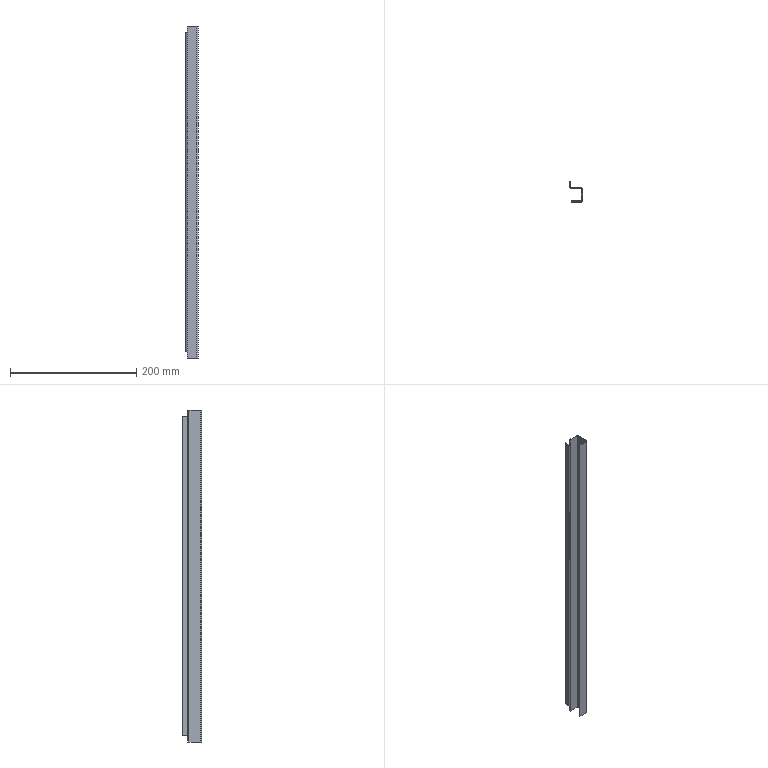Part | SolidWorks | features EdgeFlange 1, FlatPattern 1, SMBaseFlange 1, SheetMetal 1 | 1 solid | 32 faces | box 19.1 x 31.2 x 525 mm | volume 39715 mm3 | plane 26 | cylinder 6 | commonest cylinder face diameters 1.4 x3 3.8 x3
STEP:
#1=CARTESIAN_POINT('',(0.,21.2,262.5));
#2=VERTEX_POINT('',#1);
#3=CARTESIAN_POINT('',(0.,21.2,252.5));
#4=VERTEX_POINT('',#3);
#5=CARTESIAN_POINT('',(0.,21.2,262.5));
#6=DIRECTION('',(0.,0.,-1.));
#7=VECTOR('',#6,1000.);
#8=LINE('',#5,#7);
#9=EDGE_CURVE('',#2,#4,#8,.T.);
#10=ORIENTED_EDGE('',*,*,#9,.T.);
#11=CARTESIAN_POINT('',(0.,20.,252.5));
#12=VERTEX_POINT('',#11);
#13=CARTESIAN_POINT('',(0.,21.2,252.5));
#14=DIRECTION('',(0.,-1.,0.));
#15=VECTOR('',#14,1000.);
#16=LINE('',#13,#15);
#17=EDGE_CURVE('',#4,#12,#16,.T.);
#18=ORIENTED_EDGE('',*,*,#17,.T.);
#19=CARTESIAN_POINT('',(0.,20.,262.5));
#20=VERTEX_POINT('',#19);
#21=CARTESIAN_POINT('',(0.,20.,262.5));
#22=DIRECTION('',(0.,0.,-1.));
#23=VECTOR('',#22,1000.);
#24=LINE('',#21,#23);
#25=EDGE_CURVE('',#20,#12,#24,.T.);
#26=ORIENTED_EDGE('',*,*,#25,.F.);
#27=CARTESIAN_POINT('',(0.,20.,262.5));
#28=DIRECTION('',(0.,1.,0.));
#29=VECTOR('',#28,1000.);
#30=LINE('',#27,#29);
#31=EDGE_CURVE('',#20,#2,#30,.T.);
#32=ORIENTED_EDGE('',*,*,#31,.T.);
#33=EDGE_LOOP('',(#10,#18,#26,#32));
#34=FACE_OUTER_BOUND('',#33,.T.);
#35=CARTESIAN_POINT('',(0.,20.,262.5));
#36=DIRECTION('',(-1.,0.,0.));
#37=DIRECTION('',(0.,0.,1.));
#38=AXIS2_PLACEMENT_3D('',#35,#36,#37);
#39=PLANE('',#38);
#40=ADVANCED_FACE('',(#34),#39,.T.);
#41=CARTESIAN_POINT('',(16.,0.7,262.5));
#42=VERTEX_POINT('',#41);
#43=CARTESIAN_POINT('',(17.2,0.7,262.5));
#44=VERTEX_POINT('',#43);
#45=CARTESIAN_POINT('',(16.,0.7,262.5));
#46=DIRECTION('',(1.,0.,0.));
#47=VECTOR('',#46,1000.);
#48=LINE('',#45,#47);
#49=EDGE_CURVE('',#42,#44,#48,.T.);
#50=ORIENTED_EDGE('',*,*,#49,.F.);
#51=CARTESIAN_POINT('',(15.3,0.,262.5));
#52=VERTEX_POINT('',#51);
#53=CARTESIAN_POINT('',(15.3,0.7,262.5));
#54=DIRECTION('',(0.,0.,1.));
#55=DIRECTION('',(-1.,0.,0.));
#56=AXIS2_PLACEMENT_3D('',#53,#54,#55);
#57=CIRCLE('',#56,0.7);
#58=EDGE_CURVE('',#52,#42,#57,.T.);
#59=ORIENTED_EDGE('',*,*,#58,.F.);
#60=CARTESIAN_POINT('',(15.3,-1.2,262.5));
#61=VERTEX_POINT('',#60);
#62=CARTESIAN_POINT('',(15.3,-1.2,262.5));
#63=DIRECTION('',(0.,1.,0.));
#64=VECTOR('',#63,1000.);
#65=LINE('',#62,#64);
#66=EDGE_CURVE('',#61,#52,#65,.T.);
#67=ORIENTED_EDGE('',*,*,#66,.F.);
#68=CARTESIAN_POINT('',(15.3,0.7,262.5));
#69=DIRECTION('',(0.,0.,1.));
#70=DIRECTION('',(1.,0.,0.));
#71=AXIS2_PLACEMENT_3D('',#68,#69,#70);
#72=CIRCLE('',#71,1.9);
#73=EDGE_CURVE('',#61,#44,#72,.T.);
#74=ORIENTED_EDGE('',*,*,#73,.T.);
#75=EDGE_LOOP('',(#50,#59,#67,#74));
#76=FACE_OUTER_BOUND('',#75,.T.);
#77=CARTESIAN_POINT('',(16.,0.7,262.5));
#78=DIRECTION('',(0.,0.,1.));
#79=DIRECTION('',(1.,0.,0.));
#80=AXIS2_PLACEMENT_3D('',#77,#78,#79);
#81=PLANE('',#80);
#82=ADVANCED_FACE('',(#76),#81,.T.);
#83=CARTESIAN_POINT('',(16.,19.3,262.5));
#84=VERTEX_POINT('',#83);
#85=CARTESIAN_POINT('',(16.,0.,262.5));
#86=DIRECTION('',(0.,1.,0.));
#87=VECTOR('',#86,1000.);
#88=LINE('',#85,#87);
#89=EDGE_CURVE('',#42,#84,#88,.T.);
#90=ORIENTED_EDGE('',*,*,#89,.F.);
#91=ORIENTED_EDGE('',*,*,#49,.T.);
#92=CARTESIAN_POINT('',(17.2,19.3,262.5));
#93=VERTEX_POINT('',#92);
#94=CARTESIAN_POINT('',(17.2,0.,262.5));
#95=DIRECTION('',(0.,1.,0.));
#96=VECTOR('',#95,1000.);
#97=LINE('',#94,#96);
#98=EDGE_CURVE('',#44,#93,#97,.T.);
#99=ORIENTED_EDGE('',*,*,#98,.T.);
#100=CARTESIAN_POINT('',(17.2,19.3,262.5));
#101=DIRECTION('',(-1.,0.,0.));
#102=VECTOR('',#101,1000.);
#103=LINE('',#100,#102);
#104=EDGE_CURVE('',#93,#84,#103,.T.);
#105=ORIENTED_EDGE('',*,*,#104,.T.);
#106=EDGE_LOOP('',(#90,#91,#99,#105));
#107=FACE_OUTER_BOUND('',#106,.T.);
#108=CARTESIAN_POINT('',(15.3,-1.2,262.5));
#109=DIRECTION('',(0.,0.,1.));
#110=DIRECTION('',(1.,0.,0.));
#111=AXIS2_PLACEMENT_3D('',#108,#109,#110);
#112=PLANE('',#111);
#113=ADVANCED_FACE('',(#107),#112,.T.);
#114=CARTESIAN_POINT('',(15.3,0.,-262.5));
#115=VERTEX_POINT('',#114);
#116=CARTESIAN_POINT('',(15.3,-1.2,-262.5));
#117=VERTEX_POINT('',#116);
#118=CARTESIAN_POINT('',(15.3,0.,-262.5));
#119=DIRECTION('',(0.,-1.,0.));
#120=VECTOR('',#119,1000.);
#121=LINE('',#118,#120);
#122=EDGE_CURVE('',#115,#117,#121,.T.);
#123=ORIENTED_EDGE('',*,*,#122,.F.);
#124=CARTESIAN_POINT('',(16.,0.7,-262.5));
#125=VERTEX_POINT('',#124);
#126=CARTESIAN_POINT('',(15.3,0.7,-262.5));
#127=DIRECTION('',(0.,0.,1.));
#128=DIRECTION('',(-1.,0.,0.));
#129=AXIS2_PLACEMENT_3D('',#126,#127,#128);
#130=CIRCLE('',#129,0.7);
#131=EDGE_CURVE('',#115,#125,#130,.T.);
#132=ORIENTED_EDGE('',*,*,#131,.T.);
#133=CARTESIAN_POINT('',(17.2,0.7,-262.5));
#134=VERTEX_POINT('',#133);
#135=CARTESIAN_POINT('',(17.2,0.7,-262.5));
#136=DIRECTION('',(-1.,0.,0.));
#137=VECTOR('',#136,1000.);
#138=LINE('',#135,#137);
#139=EDGE_CURVE('',#134,#125,#138,.T.);
#140=ORIENTED_EDGE('',*,*,#139,.F.);
#141=CARTESIAN_POINT('',(15.3,0.7,-262.5));
#142=DIRECTION('',(0.,0.,1.));
#143=DIRECTION('',(1.,0.,0.));
#144=AXIS2_PLACEMENT_3D('',#141,#142,#143);
#145=CIRCLE('',#144,1.9);
#146=EDGE_CURVE('',#117,#134,#145,.T.);
#147=ORIENTED_EDGE('',*,*,#146,.F.);
#148=EDGE_LOOP('',(#123,#132,#140,#147));
#149=FACE_OUTER_BOUND('',#148,.T.);
#150=CARTESIAN_POINT('',(15.3,0.,-262.5));
#151=DIRECTION('',(0.,0.,-1.));
#152=DIRECTION('',(-1.,0.,0.));
#153=AXIS2_PLACEMENT_3D('',#150,#151,#152);
#154=PLANE('',#153);
#155=ADVANCED_FACE('',(#149),#154,.T.);
#156=CARTESIAN_POINT('',(0.,0.,-262.5));
#157=VERTEX_POINT('',#156);
#158=CARTESIAN_POINT('',(0.,0.,-262.5));
#159=DIRECTION('',(1.,0.,0.));
#160=VECTOR('',#159,1000.);
#161=LINE('',#158,#160);
#162=EDGE_CURVE('',#157,#115,#161,.T.);
#163=ORIENTED_EDGE('',*,*,#162,.T.);
#164=ORIENTED_EDGE('',*,*,#122,.T.);
#165=CARTESIAN_POINT('',(0.,-1.2,-262.5));
#166=VERTEX_POINT('',#165);
#167=CARTESIAN_POINT('',(0.,-1.2,-262.5));
#168=DIRECTION('',(1.,0.,0.));
#169=VECTOR('',#168,1000.);
#170=LINE('',#167,#169);
#171=EDGE_CURVE('',#166,#117,#170,.T.);
#172=ORIENTED_EDGE('',*,*,#171,.F.);
#173=CARTESIAN_POINT('',(0.,-1.2,-262.5));
#174=DIRECTION('',(0.,1.,0.));
#175=VECTOR('',#174,1000.);
#176=LINE('',#173,#175);
#177=EDGE_CURVE('',#166,#157,#176,.T.);
#178=ORIENTED_EDGE('',*,*,#177,.T.);
#179=EDGE_LOOP('',(#163,#164,#172,#178));
#180=FACE_OUTER_BOUND('',#179,.T.);
#181=CARTESIAN_POINT('',(17.2,0.7,-262.5));
#182=DIRECTION('',(0.,0.,-1.));
#183=DIRECTION('',(-1.,0.,0.));
#184=AXIS2_PLACEMENT_3D('',#181,#182,#183);
#185=PLANE('',#184);
#186=ADVANCED_FACE('',(#180),#185,.T.);
#187=CARTESIAN_POINT('',(15.3,20.,262.5));
#188=VERTEX_POINT('',#187);
#189=CARTESIAN_POINT('',(15.3,21.2,262.5));
#190=VERTEX_POINT('',#189);
#191=CARTESIAN_POINT('',(15.3,20.,262.5));
#192=DIRECTION('',(0.,1.,0.));
#193=VECTOR('',#192,1000.);
#194=LINE('',#191,#193);
#195=EDGE_CURVE('',#188,#190,#194,.T.);
#196=ORIENTED_EDGE('',*,*,#195,.F.);
#197=CARTESIAN_POINT('',(15.3,19.3,262.5));
#198=DIRECTION('',(0.,0.,1.));
#199=DIRECTION('',(-1.,0.,0.));
#200=AXIS2_PLACEMENT_3D('',#197,#198,#199);
#201=CIRCLE('',#200,0.7);
#202=EDGE_CURVE('',#84,#188,#201,.T.);
#203=ORIENTED_EDGE('',*,*,#202,.F.);
#204=ORIENTED_EDGE('',*,*,#104,.F.);
#205=CARTESIAN_POINT('',(15.3,19.3,262.5));
#206=DIRECTION('',(0.,0.,1.));
#207=DIRECTION('',(1.,0.,0.));
#208=AXIS2_PLACEMENT_3D('',#205,#206,#207);
#209=CIRCLE('',#208,1.9);
#210=EDGE_CURVE('',#93,#190,#209,.T.);
#211=ORIENTED_EDGE('',*,*,#210,.T.);
#212=EDGE_LOOP('',(#196,#203,#204,#211));
#213=FACE_OUTER_BOUND('',#212,.T.);
#214=CARTESIAN_POINT('',(15.3,20.,262.5));
#215=DIRECTION('',(0.,0.,1.));
#216=DIRECTION('',(1.,0.,0.));
#217=AXIS2_PLACEMENT_3D('',#214,#215,#216);
#218=PLANE('',#217);
#219=ADVANCED_FACE('',(#213),#218,.T.);
#220=CARTESIAN_POINT('',(16.,20.,262.5));
#221=DIRECTION('',(-1.,0.,0.));
#222=VECTOR('',#221,1000.);
#223=LINE('',#220,#222);
#224=EDGE_CURVE('',#188,#20,#223,.T.);
#225=ORIENTED_EDGE('',*,*,#224,.F.);
#226=ORIENTED_EDGE('',*,*,#195,.T.);
#227=CARTESIAN_POINT('',(16.,21.2,262.5));
#228=DIRECTION('',(-1.,0.,0.));
#229=VECTOR('',#228,1000.);
#230=LINE('',#227,#229);
#231=EDGE_CURVE('',#190,#2,#230,.T.);
#232=ORIENTED_EDGE('',*,*,#231,.T.);
#233=ORIENTED_EDGE('',*,*,#31,.F.);
#234=EDGE_LOOP('',(#225,#226,#232,#233));
#235=FACE_OUTER_BOUND('',#234,.T.);
#236=CARTESIAN_POINT('',(17.2,19.3,262.5));
#237=DIRECTION('',(0.,0.,1.));
#238=DIRECTION('',(1.,0.,0.));
#239=AXIS2_PLACEMENT_3D('',#236,#237,#238);
#240=PLANE('',#239);
#241=ADVANCED_FACE('',(#235),#240,.T.);
#242=CARTESIAN_POINT('',(16.,19.3,-262.5));
#243=VERTEX_POINT('',#242);
#244=CARTESIAN_POINT('',(17.2,19.3,-262.5));
#245=VERTEX_POINT('',#244);
#246=CARTESIAN_POINT('',(16.,19.3,-262.5));
#247=DIRECTION('',(1.,0.,0.));
#248=VECTOR('',#247,1000.);
#249=LINE('',#246,#248);
#250=EDGE_CURVE('',#243,#245,#249,.T.);
#251=ORIENTED_EDGE('',*,*,#250,.F.);
#252=CARTESIAN_POINT('',(15.3,20.,-262.5));
#253=VERTEX_POINT('',#252);
#254=CARTESIAN_POINT('',(15.3,19.3,-262.5));
#255=DIRECTION('',(0.,0.,1.));
#256=DIRECTION('',(-1.,0.,0.));
#257=AXIS2_PLACEMENT_3D('',#254,#255,#256);
#258=CIRCLE('',#257,0.7);
#259=EDGE_CURVE('',#243,#253,#258,.T.);
#260=ORIENTED_EDGE('',*,*,#259,.T.);
#261=CARTESIAN_POINT('',(15.3,21.2,-262.5));
#262=VERTEX_POINT('',#261);
#263=CARTESIAN_POINT('',(15.3,21.2,-262.5));
#264=DIRECTION('',(0.,-1.,0.));
#265=VECTOR('',#264,1000.);
#266=LINE('',#263,#265);
#267=EDGE_CURVE('',#262,#253,#266,.T.);
#268=ORIENTED_EDGE('',*,*,#267,.F.);
#269=CARTESIAN_POINT('',(15.3,19.3,-262.5));
#270=DIRECTION('',(0.,0.,1.));
#271=DIRECTION('',(1.,0.,0.));
#272=AXIS2_PLACEMENT_3D('',#269,#270,#271);
#273=CIRCLE('',#272,1.9);
#274=EDGE_CURVE('',#245,#262,#273,.T.);
#275=ORIENTED_EDGE('',*,*,#274,.F.);
#276=EDGE_LOOP('',(#251,#260,#268,#275));
#277=FACE_OUTER_BOUND('',#276,.T.);
#278=CARTESIAN_POINT('',(16.,19.3,-262.5));
#279=DIRECTION('',(0.,0.,-1.));
#280=DIRECTION('',(-1.,0.,0.));
#281=AXIS2_PLACEMENT_3D('',#278,#279,#280);
#282=PLANE('',#281);
#283=ADVANCED_FACE('',(#277),#282,.T.);
#284=CARTESIAN_POINT('',(16.,0.,-262.5));
#285=DIRECTION('',(0.,1.,0.));
#286=VECTOR('',#285,1000.);
#287=LINE('',#284,#286);
#288=EDGE_CURVE('',#125,#243,#287,.T.);
#289=ORIENTED_EDGE('',*,*,#288,.T.);
#290=ORIENTED_EDGE('',*,*,#250,.T.);
#291=CARTESIAN_POINT('',(17.2,0.,-262.5));
#292=DIRECTION('',(0.,1.,0.));
#293=VECTOR('',#292,1000.);
#294=LINE('',#291,#293);
#295=EDGE_CURVE('',#134,#245,#294,.T.);
#296=ORIENTED_EDGE('',*,*,#295,.F.);
#297=ORIENTED_EDGE('',*,*,#139,.T.);
#298=EDGE_LOOP('',(#289,#290,#296,#297));
#299=FACE_OUTER_BOUND('',#298,.T.);
#300=CARTESIAN_POINT('',(15.3,21.2,-262.5));
#301=DIRECTION('',(0.,0.,-1.));
#302=DIRECTION('',(-1.,0.,0.));
#303=AXIS2_PLACEMENT_3D('',#300,#301,#302);
#304=PLANE('',#303);
#305=ADVANCED_FACE('',(#299),#304,.T.);
#306=CARTESIAN_POINT('',(0.,21.2,-262.5));
#307=VERTEX_POINT('',#306);
#308=CARTESIAN_POINT('',(16.,21.2,-262.5));
#309=DIRECTION('',(-1.,0.,0.));
#310=VECTOR('',#309,1000.);
#311=LINE('',#308,#310);
#312=EDGE_CURVE('',#262,#307,#311,.T.);
#313=ORIENTED_EDGE('',*,*,#312,.T.);
#314=CARTESIAN_POINT('',(0.,21.2,-252.5));
#315=VERTEX_POINT('',#314);
#316=CARTESIAN_POINT('',(0.,21.2,262.5));
#317=DIRECTION('',(0.,0.,-1.));
#318=VECTOR('',#317,1000.);
#319=LINE('',#316,#318);
#320=EDGE_CURVE('',#315,#307,#319,.T.);
#321=ORIENTED_EDGE('',*,*,#320,.F.);
#322=CARTESIAN_POINT('',(0.,21.2,252.5));
#323=DIRECTION('',(0.,0.,-1.));
#324=VECTOR('',#323,1000.);
#325=LINE('',#322,#324);
#326=EDGE_CURVE('',#4,#315,#325,.T.);
#327=ORIENTED_EDGE('',*,*,#326,.F.);
#328=ORIENTED_EDGE('',*,*,#9,.F.);
#329=ORIENTED_EDGE('',*,*,#231,.F.);
#330=CARTESIAN_POINT('',(15.3,21.2,262.5));
#331=DIRECTION('',(0.,0.,-1.));
#332=VECTOR('',#331,1000.);
#333=LINE('',#330,#332);
#334=EDGE_CURVE('',#190,#262,#333,.T.);
#335=ORIENTED_EDGE('',*,*,#334,.T.);
#336=EDGE_LOOP('',(#313,#321,#327,#328,#329,#335));
#337=FACE_OUTER_BOUND('',#336,.T.);
#338=CARTESIAN_POINT('',(16.,21.2,262.5));
#339=DIRECTION('',(0.,-1.,0.));
#340=DIRECTION('',(0.,0.,-1.));
#341=AXIS2_PLACEMENT_3D('',#338,#339,#340);
#342=PLANE('',#341);
#343=ADVANCED_FACE('',(#337),#342,.F.);
#344=CARTESIAN_POINT('',(0.,20.,-252.5));
#345=VERTEX_POINT('',#344);
#346=CARTESIAN_POINT('',(0.,21.2,-252.5));
#347=DIRECTION('',(0.,-1.,0.));
#348=VECTOR('',#347,1000.);
#349=LINE('',#346,#348);
#350=EDGE_CURVE('',#315,#345,#349,.T.);
#351=ORIENTED_EDGE('',*,*,#350,.F.);
#352=ORIENTED_EDGE('',*,*,#320,.T.);
#353=CARTESIAN_POINT('',(0.,20.,-262.5));
#354=VERTEX_POINT('',#353);
#355=CARTESIAN_POINT('',(0.,20.,-262.5));
#356=DIRECTION('',(0.,1.,0.));
#357=VECTOR('',#356,1000.);
#358=LINE('',#355,#357);
#359=EDGE_CURVE('',#354,#307,#358,.T.);
#360=ORIENTED_EDGE('',*,*,#359,.F.);
#361=CARTESIAN_POINT('',(0.,20.,262.5));
#362=DIRECTION('',(0.,0.,-1.));
#363=VECTOR('',#362,1000.);
#364=LINE('',#361,#363);
#365=EDGE_CURVE('',#345,#354,#364,.T.);
#366=ORIENTED_EDGE('',*,*,#365,.F.);
#367=EDGE_LOOP('',(#351,#352,#360,#366));
#368=FACE_OUTER_BOUND('',#367,.T.);
#369=CARTESIAN_POINT('',(0.,20.,262.5));
#370=DIRECTION('',(-1.,0.,0.));
#371=DIRECTION('',(0.,0.,1.));
#372=AXIS2_PLACEMENT_3D('',#369,#370,#371);
#373=PLANE('',#372);
#374=ADVANCED_FACE('',(#368),#373,.T.);
#375=CARTESIAN_POINT('',(16.,20.,-262.5));
#376=DIRECTION('',(-1.,0.,0.));
#377=VECTOR('',#376,1000.);
#378=LINE('',#375,#377);
#379=EDGE_CURVE('',#253,#354,#378,.T.);
#380=ORIENTED_EDGE('',*,*,#379,.F.);
#381=CARTESIAN_POINT('',(15.3,20.,262.5));
#382=DIRECTION('',(0.,0.,-1.));
#383=VECTOR('',#382,1000.);
#384=LINE('',#381,#383);
#385=EDGE_CURVE('',#188,#253,#384,.T.);
#386=ORIENTED_EDGE('',*,*,#385,.F.);
#387=ORIENTED_EDGE('',*,*,#224,.T.);
#388=ORIENTED_EDGE('',*,*,#25,.T.);
#389=CARTESIAN_POINT('',(0.,20.,252.5));
#390=DIRECTION('',(0.,0.,-1.));
#391=VECTOR('',#390,1000.);
#392=LINE('',#389,#391);
#393=EDGE_CURVE('',#12,#345,#392,.T.);
#394=ORIENTED_EDGE('',*,*,#393,.T.);
#395=ORIENTED_EDGE('',*,*,#365,.T.);
#396=EDGE_LOOP('',(#380,#386,#387,#388,#394,#395));
#397=FACE_OUTER_BOUND('',#396,.T.);
#398=CARTESIAN_POINT('',(16.,20.,262.5));
#399=DIRECTION('',(0.,-1.,0.));
#400=DIRECTION('',(0.,0.,-1.));
#401=AXIS2_PLACEMENT_3D('',#398,#399,#400);
#402=PLANE('',#401);
#403=ADVANCED_FACE('',(#397),#402,.T.);
#404=ORIENTED_EDGE('',*,*,#259,.F.);
#405=CARTESIAN_POINT('',(16.,19.3,262.5));
#406=DIRECTION('',(0.,0.,-1.));
#407=VECTOR('',#406,1000.);
#408=LINE('',#405,#407);
#409=EDGE_CURVE('',#84,#243,#408,.T.);
#410=ORIENTED_EDGE('',*,*,#409,.F.);
#411=ORIENTED_EDGE('',*,*,#202,.T.);
#412=ORIENTED_EDGE('',*,*,#385,.T.);
#413=EDGE_LOOP('',(#404,#410,#411,#412));
#414=FACE_OUTER_BOUND('',#413,.T.);
#415=CARTESIAN_POINT('',(15.3,19.3,262.5));
#416=DIRECTION('',(0.,0.,-1.));
#417=DIRECTION('',(-1.,0.,0.));
#418=AXIS2_PLACEMENT_3D('',#415,#416,#417);
#419=CYLINDRICAL_SURFACE('',#418,0.7);
#420=ADVANCED_FACE('',(#414),#419,.F.);
#421=ORIENTED_EDGE('',*,*,#288,.F.);
#422=CARTESIAN_POINT('',(16.,0.7,262.5));
#423=DIRECTION('',(0.,0.,-1.));
#424=VECTOR('',#423,1000.);
#425=LINE('',#422,#424);
#426=EDGE_CURVE('',#42,#125,#425,.T.);
#427=ORIENTED_EDGE('',*,*,#426,.F.);
#428=ORIENTED_EDGE('',*,*,#89,.T.);
#429=ORIENTED_EDGE('',*,*,#409,.T.);
#430=EDGE_LOOP('',(#421,#427,#428,#429));
#431=FACE_OUTER_BOUND('',#430,.T.);
#432=CARTESIAN_POINT('',(16.,0.,262.5));
#433=DIRECTION('',(-1.,0.,0.));
#434=DIRECTION('',(0.,-1.,0.));
#435=AXIS2_PLACEMENT_3D('',#432,#433,#434);
#436=PLANE('',#435);
#437=ADVANCED_FACE('',(#431),#436,.T.);
#438=ORIENTED_EDGE('',*,*,#131,.F.);
#439=CARTESIAN_POINT('',(15.3,0.,262.5));
#440=DIRECTION('',(0.,0.,-1.));
#441=VECTOR('',#440,1000.);
#442=LINE('',#439,#441);
#443=EDGE_CURVE('',#52,#115,#442,.T.);
#444=ORIENTED_EDGE('',*,*,#443,.F.);
#445=ORIENTED_EDGE('',*,*,#58,.T.);
#446=ORIENTED_EDGE('',*,*,#426,.T.);
#447=EDGE_LOOP('',(#438,#444,#445,#446));
#448=FACE_OUTER_BOUND('',#447,.T.);
#449=CARTESIAN_POINT('',(15.3,0.7,262.5));
#450=DIRECTION('',(0.,0.,-1.));
#451=DIRECTION('',(-1.,0.,0.));
#452=AXIS2_PLACEMENT_3D('',#449,#450,#451);
#453=CYLINDRICAL_SURFACE('',#452,0.7);
#454=ADVANCED_FACE('',(#448),#453,.F.);
#455=ORIENTED_EDGE('',*,*,#162,.F.);
#456=CARTESIAN_POINT('',(0.,0.,262.5));
#457=VERTEX_POINT('',#456);
#458=CARTESIAN_POINT('',(0.,0.,262.5));
#459=DIRECTION('',(0.,0.,-1.));
#460=VECTOR('',#459,1000.);
#461=LINE('',#458,#460);
#462=EDGE_CURVE('',#457,#157,#461,.T.);
#463=ORIENTED_EDGE('',*,*,#462,.F.);
#464=CARTESIAN_POINT('',(0.,0.,262.5));
#465=DIRECTION('',(1.,0.,0.));
#466=VECTOR('',#465,1000.);
#467=LINE('',#464,#466);
#468=EDGE_CURVE('',#457,#52,#467,.T.);
#469=ORIENTED_EDGE('',*,*,#468,.T.);
#470=ORIENTED_EDGE('',*,*,#443,.T.);
#471=EDGE_LOOP('',(#455,#463,#469,#470));
#472=FACE_OUTER_BOUND('',#471,.T.);
#473=CARTESIAN_POINT('',(0.,0.,262.5));
#474=DIRECTION('',(0.,1.,0.));
#475=DIRECTION('',(-1.,0.,0.));
#476=AXIS2_PLACEMENT_3D('',#473,#474,#475);
#477=PLANE('',#476);
#478=ADVANCED_FACE('',(#472),#477,.T.);
#479=ORIENTED_EDGE('',*,*,#177,.F.);
#480=CARTESIAN_POINT('',(0.,-1.2,262.5));
#481=VERTEX_POINT('',#480);
#482=CARTESIAN_POINT('',(0.,-1.2,262.5));
#483=DIRECTION('',(0.,0.,-1.));
#484=VECTOR('',#483,1000.);
#485=LINE('',#482,#484);
#486=EDGE_CURVE('',#481,#166,#485,.T.);
#487=ORIENTED_EDGE('',*,*,#486,.F.);
#488=CARTESIAN_POINT('',(0.,-1.2,262.5));
#489=DIRECTION('',(0.,1.,0.));
#490=VECTOR('',#489,1000.);
#491=LINE('',#488,#490);
#492=EDGE_CURVE('',#481,#457,#491,.T.);
#493=ORIENTED_EDGE('',*,*,#492,.T.);
#494=ORIENTED_EDGE('',*,*,#462,.T.);
#495=EDGE_LOOP('',(#479,#487,#493,#494));
#496=FACE_OUTER_BOUND('',#495,.T.);
#497=CARTESIAN_POINT('',(0.,-1.2,262.5));
#498=DIRECTION('',(-1.,0.,0.));
#499=DIRECTION('',(0.,-1.,0.));
#500=AXIS2_PLACEMENT_3D('',#497,#498,#499);
#501=PLANE('',#500);
#502=ADVANCED_FACE('',(#496),#501,.T.);
#503=ORIENTED_EDGE('',*,*,#171,.T.);
#504=CARTESIAN_POINT('',(15.3,-1.2,262.5));
#505=DIRECTION('',(0.,0.,-1.));
#506=VECTOR('',#505,1000.);
#507=LINE('',#504,#506);
#508=EDGE_CURVE('',#61,#117,#507,.T.);
#509=ORIENTED_EDGE('',*,*,#508,.F.);
#510=CARTESIAN_POINT('',(0.,-1.2,262.5));
#511=DIRECTION('',(1.,0.,0.));
#512=VECTOR('',#511,1000.);
#513=LINE('',#510,#512);
#514=EDGE_CURVE('',#481,#61,#513,.T.);
#515=ORIENTED_EDGE('',*,*,#514,.F.);
#516=ORIENTED_EDGE('',*,*,#486,.T.);
#517=EDGE_LOOP('',(#503,#509,#515,#516));
#518=FACE_OUTER_BOUND('',#517,.T.);
#519=CARTESIAN_POINT('',(0.,-1.2,262.5));
#520=DIRECTION('',(0.,1.,0.));
#521=DIRECTION('',(-1.,0.,0.));
#522=AXIS2_PLACEMENT_3D('',#519,#520,#521);
#523=PLANE('',#522);
#524=ADVANCED_FACE('',(#518),#523,.F.);
#525=ORIENTED_EDGE('',*,*,#146,.T.);
#526=CARTESIAN_POINT('',(17.2,0.7,262.5));
#527=DIRECTION('',(0.,0.,-1.));
#528=VECTOR('',#527,1000.);
#529=LINE('',#526,#528);
#530=EDGE_CURVE('',#44,#134,#529,.T.);
#531=ORIENTED_EDGE('',*,*,#530,.F.);
#532=ORIENTED_EDGE('',*,*,#73,.F.);
#533=ORIENTED_EDGE('',*,*,#508,.T.);
#534=EDGE_LOOP('',(#525,#531,#532,#533));
#535=FACE_OUTER_BOUND('',#534,.T.);
#536=CARTESIAN_POINT('',(15.3,0.7,262.5));
#537=DIRECTION('',(0.,0.,-1.));
#538=DIRECTION('',(-1.,0.,0.));
#539=AXIS2_PLACEMENT_3D('',#536,#537,#538);
#540=CYLINDRICAL_SURFACE('',#539,1.9);
#541=ADVANCED_FACE('',(#535),#540,.T.);
#542=ORIENTED_EDGE('',*,*,#295,.T.);
#543=CARTESIAN_POINT('',(17.2,19.3,262.5));
#544=DIRECTION('',(0.,0.,-1.));
#545=VECTOR('',#544,1000.);
#546=LINE('',#543,#545);
#547=EDGE_CURVE('',#93,#245,#546,.T.);
#548=ORIENTED_EDGE('',*,*,#547,.F.);
#549=ORIENTED_EDGE('',*,*,#98,.F.);
#550=ORIENTED_EDGE('',*,*,#530,.T.);
#551=EDGE_LOOP('',(#542,#548,#549,#550));
#552=FACE_OUTER_BOUND('',#551,.T.);
#553=CARTESIAN_POINT('',(17.2,0.,262.5));
#554=DIRECTION('',(-1.,0.,0.));
#555=DIRECTION('',(0.,-1.,0.));
#556=AXIS2_PLACEMENT_3D('',#553,#554,#555);
#557=PLANE('',#556);
#558=ADVANCED_FACE('',(#552),#557,.F.);
#559=ORIENTED_EDGE('',*,*,#274,.T.);
#560=ORIENTED_EDGE('',*,*,#334,.F.);
#561=ORIENTED_EDGE('',*,*,#210,.F.);
#562=ORIENTED_EDGE('',*,*,#547,.T.);
#563=EDGE_LOOP('',(#559,#560,#561,#562));
#564=FACE_OUTER_BOUND('',#563,.T.);
#565=CARTESIAN_POINT('',(15.3,19.3,262.5));
#566=DIRECTION('',(0.,0.,-1.));
#567=DIRECTION('',(-1.,0.,0.));
#568=AXIS2_PLACEMENT_3D('',#565,#566,#567);
#569=CYLINDRICAL_SURFACE('',#568,1.9);
#570=ADVANCED_FACE('',(#564),#569,.T.);
#571=ORIENTED_EDGE('',*,*,#514,.T.);
#572=ORIENTED_EDGE('',*,*,#66,.T.);
#573=ORIENTED_EDGE('',*,*,#468,.F.);
#574=ORIENTED_EDGE('',*,*,#492,.F.);
#575=EDGE_LOOP('',(#571,#572,#573,#574));
#576=FACE_OUTER_BOUND('',#575,.T.);
#577=CARTESIAN_POINT('',(15.3,19.3,262.5));
#578=DIRECTION('',(0.,0.,-1.));
#579=DIRECTION('',(-1.,0.,0.));
#580=AXIS2_PLACEMENT_3D('',#577,#578,#579);
#581=PLANE('',#580);
#582=ADVANCED_FACE('',(#576),#581,.F.);
#583=ORIENTED_EDGE('',*,*,#312,.F.);
#584=ORIENTED_EDGE('',*,*,#267,.T.);
#585=ORIENTED_EDGE('',*,*,#379,.T.);
#586=ORIENTED_EDGE('',*,*,#359,.T.);
#587=EDGE_LOOP('',(#583,#584,#585,#586));
#588=FACE_OUTER_BOUND('',#587,.T.);
#589=CARTESIAN_POINT('',(15.3,19.3,-262.5));
#590=DIRECTION('',(0.,0.,-1.));
#591=DIRECTION('',(-1.,0.,0.));
#592=AXIS2_PLACEMENT_3D('',#589,#590,#591);
#593=PLANE('',#592);
#594=ADVANCED_FACE('',(#588),#593,.T.);
#595=CARTESIAN_POINT('',(-0.7,21.9,-252.5));
#596=VERTEX_POINT('',#595);
#597=CARTESIAN_POINT('',(-1.9,21.9,-252.5));
#598=VERTEX_POINT('',#597);
#599=CARTESIAN_POINT('',(-1.9,21.9,-252.5));
#600=DIRECTION('',(-1.,0.,0.));
#601=VECTOR('',#600,1000.);
#602=LINE('',#599,#601);
#603=EDGE_CURVE('',#596,#598,#602,.T.);
#604=ORIENTED_EDGE('',*,*,#603,.F.);
#605=CARTESIAN_POINT('',(0.,21.9,-252.5));
#606=DIRECTION('',(0.,0.,-1.));
#607=DIRECTION('',(1.,0.,0.));
#608=AXIS2_PLACEMENT_3D('',#605,#606,#607);
#609=CIRCLE('',#608,0.7);
#610=EDGE_CURVE('',#315,#596,#609,.T.);
#611=ORIENTED_EDGE('',*,*,#610,.F.);
#612=ORIENTED_EDGE('',*,*,#350,.T.);
#613=CARTESIAN_POINT('',(0.,21.9,-252.5));
#614=DIRECTION('',(0.,0.,-1.));
#615=DIRECTION('',(1.,0.,0.));
#616=AXIS2_PLACEMENT_3D('',#613,#614,#615);
#617=CIRCLE('',#616,1.9);
#618=EDGE_CURVE('',#345,#598,#617,.T.);
#619=ORIENTED_EDGE('',*,*,#618,.T.);
#620=EDGE_LOOP('',(#604,#611,#612,#619));
#621=FACE_OUTER_BOUND('',#620,.T.);
#622=CARTESIAN_POINT('',(0.,21.9,-252.5));
#623=DIRECTION('',(0.,0.,-1.));
#624=DIRECTION('',(-1.,0.,0.));
#625=AXIS2_PLACEMENT_3D('',#622,#623,#624);
#626=PLANE('',#625);
#627=ADVANCED_FACE('',(#621),#626,.T.);
#628=CARTESIAN_POINT('',(-0.7,21.9,252.5));
#629=VERTEX_POINT('',#628);
#630=CARTESIAN_POINT('',(0.,21.9,252.5));
#631=DIRECTION('',(0.,0.,1.));
#632=DIRECTION('',(1.,0.,0.));
#633=AXIS2_PLACEMENT_3D('',#630,#631,#632);
#634=CIRCLE('',#633,0.7);
#635=EDGE_CURVE('',#629,#4,#634,.T.);
#636=ORIENTED_EDGE('',*,*,#635,.F.);
#637=CARTESIAN_POINT('',(-1.9,21.9,252.5));
#638=VERTEX_POINT('',#637);
#639=CARTESIAN_POINT('',(-0.7,21.9,252.5));
#640=DIRECTION('',(-1.,0.,0.));
#641=VECTOR('',#640,1000.);
#642=LINE('',#639,#641);
#643=EDGE_CURVE('',#629,#638,#642,.T.);
#644=ORIENTED_EDGE('',*,*,#643,.T.);
#645=CARTESIAN_POINT('',(0.,21.9,252.5));
#646=DIRECTION('',(0.,0.,1.));
#647=DIRECTION('',(1.,0.,0.));
#648=AXIS2_PLACEMENT_3D('',#645,#646,#647);
#649=CIRCLE('',#648,1.9);
#650=EDGE_CURVE('',#638,#12,#649,.T.);
#651=ORIENTED_EDGE('',*,*,#650,.T.);
#652=ORIENTED_EDGE('',*,*,#17,.F.);
#653=EDGE_LOOP('',(#636,#644,#651,#652));
#654=FACE_OUTER_BOUND('',#653,.T.);
#655=CARTESIAN_POINT('',(0.,21.9,252.5));
#656=DIRECTION('',(0.,0.,-1.));
#657=DIRECTION('',(-1.,0.,0.));
#658=AXIS2_PLACEMENT_3D('',#655,#656,#657);
#659=PLANE('',#658);
#660=ADVANCED_FACE('',(#654),#659,.F.);
#661=ORIENTED_EDGE('',*,*,#393,.F.);
#662=ORIENTED_EDGE('',*,*,#650,.F.);
#663=CARTESIAN_POINT('',(-1.9,21.9,-252.5));
#664=DIRECTION('',(0.,0.,-1.));
#665=VECTOR('',#664,1000.);
#666=LINE('',#663,#665);
#667=EDGE_CURVE('',#638,#598,#666,.T.);
#668=ORIENTED_EDGE('',*,*,#667,.T.);
#669=ORIENTED_EDGE('',*,*,#618,.F.);
#670=EDGE_LOOP('',(#661,#662,#668,#669));
#671=FACE_OUTER_BOUND('',#670,.T.);
#672=CARTESIAN_POINT('',(0.,21.9,252.5));
#673=DIRECTION('',(0.,0.,1.));
#674=DIRECTION('',(-1.,0.,0.));
#675=AXIS2_PLACEMENT_3D('',#672,#673,#674);
#676=CYLINDRICAL_SURFACE('',#675,1.9);
#677=ADVANCED_FACE('',(#671),#676,.T.);
#678=ORIENTED_EDGE('',*,*,#326,.T.);
#679=ORIENTED_EDGE('',*,*,#610,.T.);
#680=CARTESIAN_POINT('',(-0.7,21.9,-252.5));
#681=DIRECTION('',(0.,0.,1.));
#682=VECTOR('',#681,1000.);
#683=LINE('',#680,#682);
#684=EDGE_CURVE('',#596,#629,#683,.T.);
#685=ORIENTED_EDGE('',*,*,#684,.T.);
#686=ORIENTED_EDGE('',*,*,#635,.T.);
#687=EDGE_LOOP('',(#678,#679,#685,#686));
#688=FACE_OUTER_BOUND('',#687,.T.);
#689=CARTESIAN_POINT('',(0.,21.9,252.5));
#690=DIRECTION('',(0.,0.,1.));
#691=DIRECTION('',(-1.,0.,0.));
#692=AXIS2_PLACEMENT_3D('',#689,#690,#691);
#693=CYLINDRICAL_SURFACE('',#692,0.7);
#694=ADVANCED_FACE('',(#688),#693,.F.);
#695=ORIENTED_EDGE('',*,*,#643,.F.);
#696=CARTESIAN_POINT('',(-0.7,30.,252.5));
#697=VERTEX_POINT('',#696);
#698=CARTESIAN_POINT('',(-0.7,30.,252.5));
#699=DIRECTION('',(0.,1.,0.));
#700=VECTOR('',#699,1000.);
#701=LINE('',#698,#700);
#702=EDGE_CURVE('',#629,#697,#701,.T.);
#703=ORIENTED_EDGE('',*,*,#702,.T.);
#704=CARTESIAN_POINT('',(-1.9,30.,252.5));
#705=VERTEX_POINT('',#704);
#706=CARTESIAN_POINT('',(-1.9,30.,252.5));
#707=DIRECTION('',(1.,0.,0.));
#708=VECTOR('',#707,1000.);
#709=LINE('',#706,#708);
#710=EDGE_CURVE('',#705,#697,#709,.T.);
#711=ORIENTED_EDGE('',*,*,#710,.F.);
#712=CARTESIAN_POINT('',(-1.9,0.,252.5));
#713=DIRECTION('',(0.,1.,0.));
#714=VECTOR('',#713,1000.);
#715=LINE('',#712,#714);
#716=EDGE_CURVE('',#638,#705,#715,.T.);
#717=ORIENTED_EDGE('',*,*,#716,.F.);
#718=EDGE_LOOP('',(#695,#703,#711,#717));
#719=FACE_OUTER_BOUND('',#718,.T.);
#720=CARTESIAN_POINT('',(-1.9,30.,252.5));
#721=DIRECTION('',(0.,0.,-1.));
#722=DIRECTION('',(-1.,0.,0.));
#723=AXIS2_PLACEMENT_3D('',#720,#721,#722);
#724=PLANE('',#723);
#725=ADVANCED_FACE('',(#719),#724,.F.);
#726=ORIENTED_EDGE('',*,*,#603,.T.);
#727=CARTESIAN_POINT('',(-1.9,30.,-252.5));
#728=VERTEX_POINT('',#727);
#729=CARTESIAN_POINT('',(-1.9,0.,-252.5));
#730=DIRECTION('',(0.,-1.,0.));
#731=VECTOR('',#730,1000.);
#732=LINE('',#729,#731);
#733=EDGE_CURVE('',#728,#598,#732,.T.);
#734=ORIENTED_EDGE('',*,*,#733,.F.);
#735=CARTESIAN_POINT('',(-0.7,30.,-252.5));
#736=VERTEX_POINT('',#735);
#737=CARTESIAN_POINT('',(-1.9,30.,-252.5));
#738=DIRECTION('',(1.,0.,0.));
#739=VECTOR('',#738,1000.);
#740=LINE('',#737,#739);
#741=EDGE_CURVE('',#728,#736,#740,.T.);
#742=ORIENTED_EDGE('',*,*,#741,.T.);
#743=CARTESIAN_POINT('',(-0.7,21.2,-252.5));
#744=DIRECTION('',(0.,-1.,0.));
#745=VECTOR('',#744,1000.);
#746=LINE('',#743,#745);
#747=EDGE_CURVE('',#736,#596,#746,.T.);
#748=ORIENTED_EDGE('',*,*,#747,.T.);
#749=EDGE_LOOP('',(#726,#734,#742,#748));
#750=FACE_OUTER_BOUND('',#749,.T.);
#751=CARTESIAN_POINT('',(-1.9,21.2,-252.5));
#752=DIRECTION('',(0.,0.,1.));
#753=DIRECTION('',(0.,-1.,0.));
#754=AXIS2_PLACEMENT_3D('',#751,#752,#753);
#755=PLANE('',#754);
#756=ADVANCED_FACE('',(#750),#755,.F.);
#757=ORIENTED_EDGE('',*,*,#667,.F.);
#758=ORIENTED_EDGE('',*,*,#716,.T.);
#759=CARTESIAN_POINT('',(-1.9,30.,0.));
#760=DIRECTION('',(0.,0.,-1.));
#761=VECTOR('',#760,1000.);
#762=LINE('',#759,#761);
#763=EDGE_CURVE('',#705,#728,#762,.T.);
#764=ORIENTED_EDGE('',*,*,#763,.T.);
#765=ORIENTED_EDGE('',*,*,#733,.T.);
#766=EDGE_LOOP('',(#757,#758,#764,#765));
#767=FACE_OUTER_BOUND('',#766,.T.);
#768=CARTESIAN_POINT('',(-1.9,0.,0.));
#769=DIRECTION('',(1.,0.,0.));
#770=DIRECTION('',(0.,1.,0.));
#771=AXIS2_PLACEMENT_3D('',#768,#769,#770);
#772=PLANE('',#771);
#773=ADVANCED_FACE('',(#767),#772,.F.);
#774=ORIENTED_EDGE('',*,*,#702,.F.);
#775=ORIENTED_EDGE('',*,*,#684,.F.);
#776=ORIENTED_EDGE('',*,*,#747,.F.);
#777=CARTESIAN_POINT('',(-0.7,30.,-252.5));
#778=DIRECTION('',(0.,0.,-1.));
#779=VECTOR('',#778,1000.);
#780=LINE('',#777,#779);
#781=EDGE_CURVE('',#697,#736,#780,.T.);
#782=ORIENTED_EDGE('',*,*,#781,.F.);
#783=EDGE_LOOP('',(#774,#775,#776,#782));
#784=FACE_OUTER_BOUND('',#783,.T.);
#785=CARTESIAN_POINT('',(-0.7,0.,0.));
#786=DIRECTION('',(1.,0.,0.));
#787=DIRECTION('',(0.,1.,0.));
#788=AXIS2_PLACEMENT_3D('',#785,#786,#787);
#789=PLANE('',#788);
#790=ADVANCED_FACE('',(#784),#789,.T.);
#791=ORIENTED_EDGE('',*,*,#781,.T.);
#792=ORIENTED_EDGE('',*,*,#741,.F.);
#793=ORIENTED_EDGE('',*,*,#763,.F.);
#794=ORIENTED_EDGE('',*,*,#710,.T.);
#795=EDGE_LOOP('',(#791,#792,#793,#794));
#796=FACE_OUTER_BOUND('',#795,.T.);
#797=CARTESIAN_POINT('',(-1.9,30.,-252.5));
#798=DIRECTION('',(0.,-1.,0.));
#799=DIRECTION('',(1.,0.,0.));
#800=AXIS2_PLACEMENT_3D('',#797,#798,#799);
#801=PLANE('',#800);
#802=ADVANCED_FACE('',(#796),#801,.F.);
#803=CLOSED_SHELL('',(#40,#82,#113,#155,#186,#219,#241,#283,#305,#343,#374,#403,#420,#437,#454,#478,#502,#524,#541,#558,#570,#582,#594,#627,#660,#677,#694,#725,#756,#773,#790,#802));
#804=MANIFOLD_SOLID_BREP('',#803);
#805=CARTESIAN_POINT('',(0.,0.,0.));
#806=DIRECTION('',(0.,0.,1.));
#807=DIRECTION('',(1.,0.,0.));
#808=AXIS2_PLACEMENT_3D('',#805,#806,#807);
#809=(LENGTH_UNIT()NAMED_UNIT(*)SI_UNIT(.MILLI.,.METRE.));
#810=UNCERTAINTY_MEASURE_WITH_UNIT(LENGTH_MEASURE(0.00001),#809,'','');
#811=(NAMED_UNIT(*)PLANE_ANGLE_UNIT()SI_UNIT($,.RADIAN.));
#812=(NAMED_UNIT(*)SI_UNIT($,.STERADIAN.)SOLID_ANGLE_UNIT());
#813=(GEOMETRIC_REPRESENTATION_CONTEXT(3)GLOBAL_UNCERTAINTY_ASSIGNED_CONTEXT((#810))GLOBAL_UNIT_ASSIGNED_CONTEXT((#809,#811,#812))REPRESENTATION_CONTEXT('',''));
#814=ADVANCED_BREP_SHAPE_REPRESENTATION('',(#804,#808),#813);